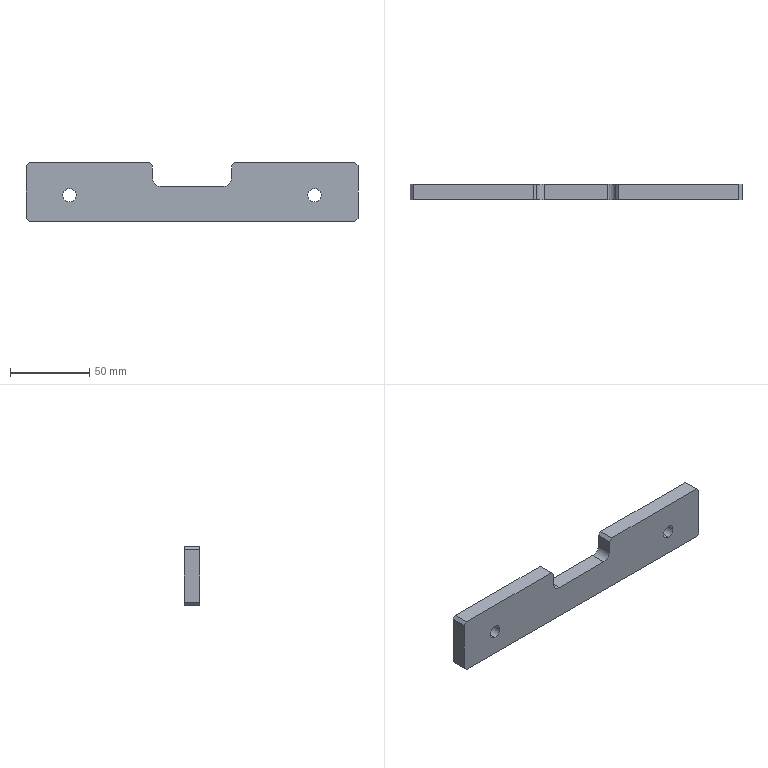Part | STEP file | PN_0016 Cylinder Plate_Default | 1 solid | 22 faces | box 210 x 10 x 37 mm | volume 69052 mm3 | plane 16 | cylinder 6 | commonest cylinder face diameters 8.5 x4 10 x2